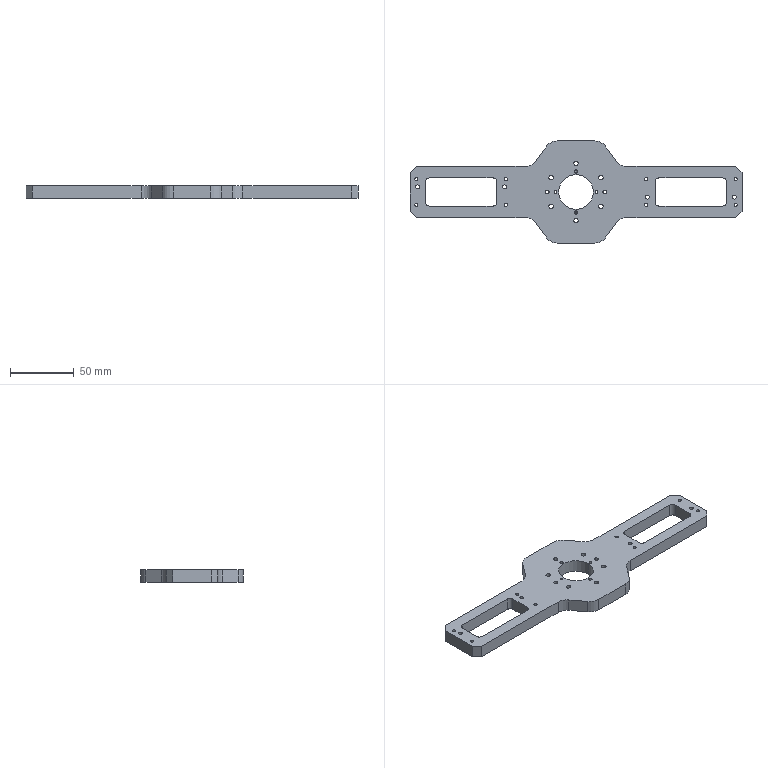Part | 1 solid | 96 faces | box 259.7 x 80 x 10 mm | volume 93464 mm3 | cylinder 66 | plane 26 | cone 4 | commonest cylinder face diameters 2.5 x20 3 x12 3.5 x12 6 x8 20 x8 2 x4